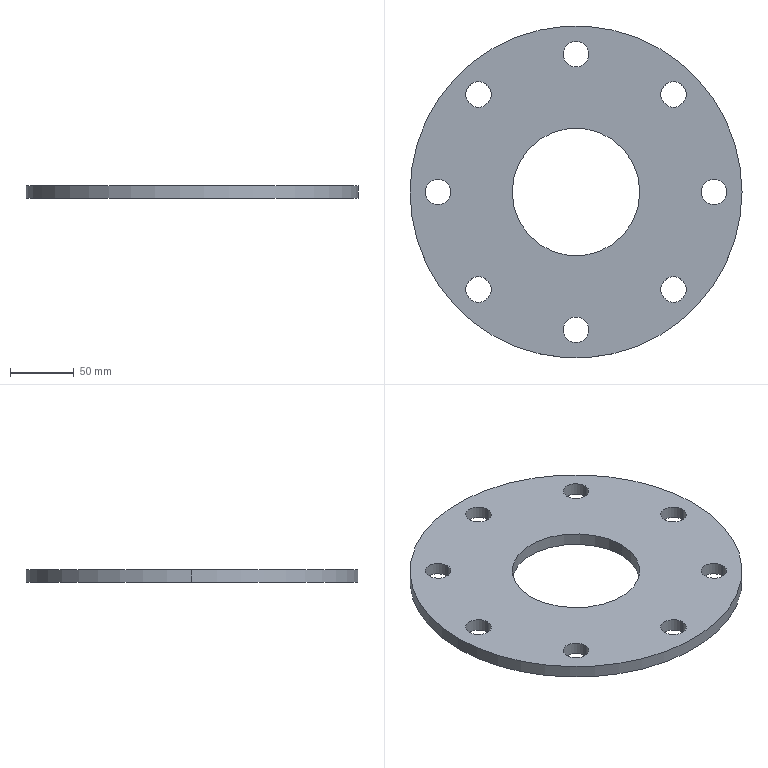Part | SolidWorks | features Extrusion 1, ICE 1 | 1 solid | 22 faces | box 260 x 260 x 10 mm | volume 427257 mm3 | cylinder 20 | plane 2 | commonest cylinder face diameters 20 x16 100 x2 260 x2
STEP:
#1=CARTESIAN_POINT('',(-50.,0.,-5.));
#2=VERTEX_POINT('',#1);
#3=CARTESIAN_POINT('',(50.,0.,-5.));
#4=VERTEX_POINT('',#3);
#5=CARTESIAN_POINT('',(0.,0.,-5.));
#6=DIRECTION('',(0.,0.,1.));
#7=DIRECTION('',(1.,0.,0.));
#8=AXIS2_PLACEMENT_3D('',#5,#6,#7);
#9=CIRCLE('',#8,50.);
#10=EDGE_CURVE('',#2,#4,#9,.T.);
#11=ORIENTED_EDGE('',*,*,#10,.F.);
#12=CARTESIAN_POINT('',(-50.,0.,5.));
#13=VERTEX_POINT('',#12);
#14=CARTESIAN_POINT('',(-50.,0.,-5.));
#15=DIRECTION('',(0.,0.,1.));
#16=VECTOR('',#15,1000.);
#17=LINE('',#14,#16);
#18=EDGE_CURVE('',#2,#13,#17,.T.);
#19=ORIENTED_EDGE('',*,*,#18,.T.);
#20=CARTESIAN_POINT('',(50.,0.,5.));
#21=VERTEX_POINT('',#20);
#22=CARTESIAN_POINT('',(0.,0.,5.));
#23=DIRECTION('',(0.,0.,1.));
#24=DIRECTION('',(1.,0.,0.));
#25=AXIS2_PLACEMENT_3D('',#22,#23,#24);
#26=CIRCLE('',#25,50.);
#27=EDGE_CURVE('',#13,#21,#26,.T.);
#28=ORIENTED_EDGE('',*,*,#27,.T.);
#29=CARTESIAN_POINT('',(50.,0.,-5.));
#30=DIRECTION('',(0.,0.,1.));
#31=VECTOR('',#30,1000.);
#32=LINE('',#29,#31);
#33=EDGE_CURVE('',#4,#21,#32,.T.);
#34=ORIENTED_EDGE('',*,*,#33,.F.);
#35=EDGE_LOOP('',(#11,#19,#28,#34));
#36=FACE_OUTER_BOUND('',#35,.T.);
#37=CARTESIAN_POINT('',(0.,0.,-5.));
#38=DIRECTION('',(0.,0.,1.));
#39=DIRECTION('',(1.,0.,0.));
#40=AXIS2_PLACEMENT_3D('',#37,#38,#39);
#41=CYLINDRICAL_SURFACE('',#40,50.);
#42=ADVANCED_FACE('',(#36),#41,.F.);
#43=CARTESIAN_POINT('',(-86.368,76.368,5.));
#44=VERTEX_POINT('',#43);
#45=CARTESIAN_POINT('',(-66.368,76.368,5.));
#46=VERTEX_POINT('',#45);
#47=CARTESIAN_POINT('',(-76.368,76.368,5.));
#48=DIRECTION('',(0.,0.,1.));
#49=DIRECTION('',(1.,0.,0.));
#50=AXIS2_PLACEMENT_3D('',#47,#48,#49);
#51=CIRCLE('',#50,10.);
#52=EDGE_CURVE('',#44,#46,#51,.T.);
#53=ORIENTED_EDGE('',*,*,#52,.T.);
#54=CARTESIAN_POINT('',(-66.368,76.368,-5.));
#55=VERTEX_POINT('',#54);
#56=CARTESIAN_POINT('',(-66.368,76.368,5.));
#57=DIRECTION('',(0.,0.,-1.));
#58=VECTOR('',#57,1000.);
#59=LINE('',#56,#58);
#60=EDGE_CURVE('',#46,#55,#59,.T.);
#61=ORIENTED_EDGE('',*,*,#60,.T.);
#62=CARTESIAN_POINT('',(-86.368,76.368,-5.));
#63=VERTEX_POINT('',#62);
#64=CARTESIAN_POINT('',(-76.368,76.368,-5.));
#65=DIRECTION('',(0.,0.,1.));
#66=DIRECTION('',(1.,0.,0.));
#67=AXIS2_PLACEMENT_3D('',#64,#65,#66);
#68=CIRCLE('',#67,10.);
#69=EDGE_CURVE('',#63,#55,#68,.T.);
#70=ORIENTED_EDGE('',*,*,#69,.F.);
#71=CARTESIAN_POINT('',(-86.368,76.368,5.));
#72=DIRECTION('',(0.,0.,-1.));
#73=VECTOR('',#72,1000.);
#74=LINE('',#71,#73);
#75=EDGE_CURVE('',#44,#63,#74,.T.);
#76=ORIENTED_EDGE('',*,*,#75,.F.);
#77=EDGE_LOOP('',(#53,#61,#70,#76));
#78=FACE_OUTER_BOUND('',#77,.T.);
#79=CARTESIAN_POINT('',(-76.368,76.368,5.));
#80=DIRECTION('',(0.,0.,-1.));
#81=DIRECTION('',(-1.,0.,0.));
#82=AXIS2_PLACEMENT_3D('',#79,#80,#81);
#83=CYLINDRICAL_SURFACE('',#82,10.);
#84=ADVANCED_FACE('',(#78),#83,.F.);
#85=CARTESIAN_POINT('',(-118.,0.,5.));
#86=VERTEX_POINT('',#85);
#87=CARTESIAN_POINT('',(-98.,0.,5.));
#88=VERTEX_POINT('',#87);
#89=CARTESIAN_POINT('',(-108.,0.,5.));
#90=DIRECTION('',(0.,0.,1.));
#91=DIRECTION('',(1.,0.,0.));
#92=AXIS2_PLACEMENT_3D('',#89,#90,#91);
#93=CIRCLE('',#92,10.);
#94=EDGE_CURVE('',#86,#88,#93,.T.);
#95=ORIENTED_EDGE('',*,*,#94,.T.);
#96=CARTESIAN_POINT('',(-98.,0.,-5.));
#97=VERTEX_POINT('',#96);
#98=CARTESIAN_POINT('',(-98.,0.,5.));
#99=DIRECTION('',(0.,0.,-1.));
#100=VECTOR('',#99,1000.);
#101=LINE('',#98,#100);
#102=EDGE_CURVE('',#88,#97,#101,.T.);
#103=ORIENTED_EDGE('',*,*,#102,.T.);
#104=CARTESIAN_POINT('',(-118.,0.,-5.));
#105=VERTEX_POINT('',#104);
#106=CARTESIAN_POINT('',(-108.,0.,-5.));
#107=DIRECTION('',(0.,0.,1.));
#108=DIRECTION('',(1.,0.,0.));
#109=AXIS2_PLACEMENT_3D('',#106,#107,#108);
#110=CIRCLE('',#109,10.);
#111=EDGE_CURVE('',#105,#97,#110,.T.);
#112=ORIENTED_EDGE('',*,*,#111,.F.);
#113=CARTESIAN_POINT('',(-118.,0.,5.));
#114=DIRECTION('',(0.,0.,-1.));
#115=VECTOR('',#114,1000.);
#116=LINE('',#113,#115);
#117=EDGE_CURVE('',#86,#105,#116,.T.);
#118=ORIENTED_EDGE('',*,*,#117,.F.);
#119=EDGE_LOOP('',(#95,#103,#112,#118));
#120=FACE_OUTER_BOUND('',#119,.T.);
#121=CARTESIAN_POINT('',(-108.,0.,5.));
#122=DIRECTION('',(0.,0.,-1.));
#123=DIRECTION('',(-1.,0.,0.));
#124=AXIS2_PLACEMENT_3D('',#121,#122,#123);
#125=CYLINDRICAL_SURFACE('',#124,10.);
#126=ADVANCED_FACE('',(#120),#125,.F.);
#127=CARTESIAN_POINT('',(-86.368,-76.368,5.));
#128=VERTEX_POINT('',#127);
#129=CARTESIAN_POINT('',(-66.368,-76.368,5.));
#130=VERTEX_POINT('',#129);
#131=CARTESIAN_POINT('',(-76.368,-76.368,5.));
#132=DIRECTION('',(0.,0.,1.));
#133=DIRECTION('',(1.,0.,0.));
#134=AXIS2_PLACEMENT_3D('',#131,#132,#133);
#135=CIRCLE('',#134,10.);
#136=EDGE_CURVE('',#128,#130,#135,.T.);
#137=ORIENTED_EDGE('',*,*,#136,.T.);
#138=CARTESIAN_POINT('',(-66.368,-76.368,-5.));
#139=VERTEX_POINT('',#138);
#140=CARTESIAN_POINT('',(-66.368,-76.368,5.));
#141=DIRECTION('',(0.,0.,-1.));
#142=VECTOR('',#141,1000.);
#143=LINE('',#140,#142);
#144=EDGE_CURVE('',#130,#139,#143,.T.);
#145=ORIENTED_EDGE('',*,*,#144,.T.);
#146=CARTESIAN_POINT('',(-86.368,-76.368,-5.));
#147=VERTEX_POINT('',#146);
#148=CARTESIAN_POINT('',(-76.368,-76.368,-5.));
#149=DIRECTION('',(0.,0.,1.));
#150=DIRECTION('',(1.,0.,0.));
#151=AXIS2_PLACEMENT_3D('',#148,#149,#150);
#152=CIRCLE('',#151,10.);
#153=EDGE_CURVE('',#147,#139,#152,.T.);
#154=ORIENTED_EDGE('',*,*,#153,.F.);
#155=CARTESIAN_POINT('',(-86.368,-76.368,5.));
#156=DIRECTION('',(0.,0.,-1.));
#157=VECTOR('',#156,1000.);
#158=LINE('',#155,#157);
#159=EDGE_CURVE('',#128,#147,#158,.T.);
#160=ORIENTED_EDGE('',*,*,#159,.F.);
#161=EDGE_LOOP('',(#137,#145,#154,#160));
#162=FACE_OUTER_BOUND('',#161,.T.);
#163=CARTESIAN_POINT('',(-76.368,-76.368,5.));
#164=DIRECTION('',(0.,0.,-1.));
#165=DIRECTION('',(-1.,0.,0.));
#166=AXIS2_PLACEMENT_3D('',#163,#164,#165);
#167=CYLINDRICAL_SURFACE('',#166,10.);
#168=ADVANCED_FACE('',(#162),#167,.F.);
#169=CARTESIAN_POINT('',(-10.,-108.,5.));
#170=VERTEX_POINT('',#169);
#171=CARTESIAN_POINT('',(10.,-108.,5.));
#172=VERTEX_POINT('',#171);
#173=CARTESIAN_POINT('',(0.,-108.,5.));
#174=DIRECTION('',(0.,0.,1.));
#175=DIRECTION('',(1.,0.,0.));
#176=AXIS2_PLACEMENT_3D('',#173,#174,#175);
#177=CIRCLE('',#176,10.);
#178=EDGE_CURVE('',#170,#172,#177,.T.);
#179=ORIENTED_EDGE('',*,*,#178,.T.);
#180=CARTESIAN_POINT('',(10.,-108.,-5.));
#181=VERTEX_POINT('',#180);
#182=CARTESIAN_POINT('',(10.,-108.,5.));
#183=DIRECTION('',(0.,0.,-1.));
#184=VECTOR('',#183,1000.);
#185=LINE('',#182,#184);
#186=EDGE_CURVE('',#172,#181,#185,.T.);
#187=ORIENTED_EDGE('',*,*,#186,.T.);
#188=CARTESIAN_POINT('',(-10.,-108.,-5.));
#189=VERTEX_POINT('',#188);
#190=CARTESIAN_POINT('',(0.,-108.,-5.));
#191=DIRECTION('',(0.,0.,1.));
#192=DIRECTION('',(1.,0.,0.));
#193=AXIS2_PLACEMENT_3D('',#190,#191,#192);
#194=CIRCLE('',#193,10.);
#195=EDGE_CURVE('',#189,#181,#194,.T.);
#196=ORIENTED_EDGE('',*,*,#195,.F.);
#197=CARTESIAN_POINT('',(-10.,-108.,5.));
#198=DIRECTION('',(0.,0.,-1.));
#199=VECTOR('',#198,1000.);
#200=LINE('',#197,#199);
#201=EDGE_CURVE('',#170,#189,#200,.T.);
#202=ORIENTED_EDGE('',*,*,#201,.F.);
#203=EDGE_LOOP('',(#179,#187,#196,#202));
#204=FACE_OUTER_BOUND('',#203,.T.);
#205=CARTESIAN_POINT('',(0.,-108.,5.));
#206=DIRECTION('',(0.,0.,-1.));
#207=DIRECTION('',(-1.,0.,0.));
#208=AXIS2_PLACEMENT_3D('',#205,#206,#207);
#209=CYLINDRICAL_SURFACE('',#208,10.);
#210=ADVANCED_FACE('',(#204),#209,.F.);
#211=CARTESIAN_POINT('',(66.368,-76.368,5.));
#212=VERTEX_POINT('',#211);
#213=CARTESIAN_POINT('',(86.368,-76.368,5.));
#214=VERTEX_POINT('',#213);
#215=CARTESIAN_POINT('',(76.368,-76.368,5.));
#216=DIRECTION('',(0.,0.,1.));
#217=DIRECTION('',(1.,0.,0.));
#218=AXIS2_PLACEMENT_3D('',#215,#216,#217);
#219=CIRCLE('',#218,10.);
#220=EDGE_CURVE('',#212,#214,#219,.T.);
#221=ORIENTED_EDGE('',*,*,#220,.T.);
#222=CARTESIAN_POINT('',(86.368,-76.368,-5.));
#223=VERTEX_POINT('',#222);
#224=CARTESIAN_POINT('',(86.368,-76.368,5.));
#225=DIRECTION('',(0.,0.,-1.));
#226=VECTOR('',#225,1000.);
#227=LINE('',#224,#226);
#228=EDGE_CURVE('',#214,#223,#227,.T.);
#229=ORIENTED_EDGE('',*,*,#228,.T.);
#230=CARTESIAN_POINT('',(66.368,-76.368,-5.));
#231=VERTEX_POINT('',#230);
#232=CARTESIAN_POINT('',(76.368,-76.368,-5.));
#233=DIRECTION('',(0.,0.,1.));
#234=DIRECTION('',(1.,0.,0.));
#235=AXIS2_PLACEMENT_3D('',#232,#233,#234);
#236=CIRCLE('',#235,10.);
#237=EDGE_CURVE('',#231,#223,#236,.T.);
#238=ORIENTED_EDGE('',*,*,#237,.F.);
#239=CARTESIAN_POINT('',(66.368,-76.368,5.));
#240=DIRECTION('',(0.,0.,-1.));
#241=VECTOR('',#240,1000.);
#242=LINE('',#239,#241);
#243=EDGE_CURVE('',#212,#231,#242,.T.);
#244=ORIENTED_EDGE('',*,*,#243,.F.);
#245=EDGE_LOOP('',(#221,#229,#238,#244));
#246=FACE_OUTER_BOUND('',#245,.T.);
#247=CARTESIAN_POINT('',(76.368,-76.368,5.));
#248=DIRECTION('',(0.,0.,-1.));
#249=DIRECTION('',(-1.,0.,0.));
#250=AXIS2_PLACEMENT_3D('',#247,#248,#249);
#251=CYLINDRICAL_SURFACE('',#250,10.);
#252=ADVANCED_FACE('',(#246),#251,.F.);
#253=CARTESIAN_POINT('',(98.,0.,5.));
#254=VERTEX_POINT('',#253);
#255=CARTESIAN_POINT('',(118.,0.,5.));
#256=VERTEX_POINT('',#255);
#257=CARTESIAN_POINT('',(108.,0.,5.));
#258=DIRECTION('',(0.,0.,1.));
#259=DIRECTION('',(1.,0.,0.));
#260=AXIS2_PLACEMENT_3D('',#257,#258,#259);
#261=CIRCLE('',#260,10.);
#262=EDGE_CURVE('',#254,#256,#261,.T.);
#263=ORIENTED_EDGE('',*,*,#262,.T.);
#264=CARTESIAN_POINT('',(118.,0.,-5.));
#265=VERTEX_POINT('',#264);
#266=CARTESIAN_POINT('',(118.,0.,5.));
#267=DIRECTION('',(0.,0.,-1.));
#268=VECTOR('',#267,1000.);
#269=LINE('',#266,#268);
#270=EDGE_CURVE('',#256,#265,#269,.T.);
#271=ORIENTED_EDGE('',*,*,#270,.T.);
#272=CARTESIAN_POINT('',(98.,0.,-5.));
#273=VERTEX_POINT('',#272);
#274=CARTESIAN_POINT('',(108.,0.,-5.));
#275=DIRECTION('',(0.,0.,1.));
#276=DIRECTION('',(1.,0.,0.));
#277=AXIS2_PLACEMENT_3D('',#274,#275,#276);
#278=CIRCLE('',#277,10.);
#279=EDGE_CURVE('',#273,#265,#278,.T.);
#280=ORIENTED_EDGE('',*,*,#279,.F.);
#281=CARTESIAN_POINT('',(98.,0.,5.));
#282=DIRECTION('',(0.,0.,-1.));
#283=VECTOR('',#282,1000.);
#284=LINE('',#281,#283);
#285=EDGE_CURVE('',#254,#273,#284,.T.);
#286=ORIENTED_EDGE('',*,*,#285,.F.);
#287=EDGE_LOOP('',(#263,#271,#280,#286));
#288=FACE_OUTER_BOUND('',#287,.T.);
#289=CARTESIAN_POINT('',(108.,0.,5.));
#290=DIRECTION('',(0.,0.,-1.));
#291=DIRECTION('',(-1.,0.,0.));
#292=AXIS2_PLACEMENT_3D('',#289,#290,#291);
#293=CYLINDRICAL_SURFACE('',#292,10.);
#294=ADVANCED_FACE('',(#288),#293,.F.);
#295=CARTESIAN_POINT('',(66.368,76.368,5.));
#296=VERTEX_POINT('',#295);
#297=CARTESIAN_POINT('',(86.368,76.368,5.));
#298=VERTEX_POINT('',#297);
#299=CARTESIAN_POINT('',(76.368,76.368,5.));
#300=DIRECTION('',(0.,0.,1.));
#301=DIRECTION('',(1.,0.,0.));
#302=AXIS2_PLACEMENT_3D('',#299,#300,#301);
#303=CIRCLE('',#302,10.);
#304=EDGE_CURVE('',#296,#298,#303,.T.);
#305=ORIENTED_EDGE('',*,*,#304,.T.);
#306=CARTESIAN_POINT('',(86.368,76.368,-5.));
#307=VERTEX_POINT('',#306);
#308=CARTESIAN_POINT('',(86.368,76.368,5.));
#309=DIRECTION('',(0.,0.,-1.));
#310=VECTOR('',#309,1000.);
#311=LINE('',#308,#310);
#312=EDGE_CURVE('',#298,#307,#311,.T.);
#313=ORIENTED_EDGE('',*,*,#312,.T.);
#314=CARTESIAN_POINT('',(66.368,76.368,-5.));
#315=VERTEX_POINT('',#314);
#316=CARTESIAN_POINT('',(76.368,76.368,-5.));
#317=DIRECTION('',(0.,0.,1.));
#318=DIRECTION('',(1.,0.,0.));
#319=AXIS2_PLACEMENT_3D('',#316,#317,#318);
#320=CIRCLE('',#319,10.);
#321=EDGE_CURVE('',#315,#307,#320,.T.);
#322=ORIENTED_EDGE('',*,*,#321,.F.);
#323=CARTESIAN_POINT('',(66.368,76.368,5.));
#324=DIRECTION('',(0.,0.,-1.));
#325=VECTOR('',#324,1000.);
#326=LINE('',#323,#325);
#327=EDGE_CURVE('',#296,#315,#326,.T.);
#328=ORIENTED_EDGE('',*,*,#327,.F.);
#329=EDGE_LOOP('',(#305,#313,#322,#328));
#330=FACE_OUTER_BOUND('',#329,.T.);
#331=CARTESIAN_POINT('',(76.368,76.368,5.));
#332=DIRECTION('',(0.,0.,-1.));
#333=DIRECTION('',(-1.,0.,0.));
#334=AXIS2_PLACEMENT_3D('',#331,#332,#333);
#335=CYLINDRICAL_SURFACE('',#334,10.);
#336=ADVANCED_FACE('',(#330),#335,.F.);
#337=CARTESIAN_POINT('',(-10.,108.,5.));
#338=VERTEX_POINT('',#337);
#339=CARTESIAN_POINT('',(10.,108.,5.));
#340=VERTEX_POINT('',#339);
#341=CARTESIAN_POINT('',(0.,108.,5.));
#342=DIRECTION('',(0.,0.,1.));
#343=DIRECTION('',(1.,0.,0.));
#344=AXIS2_PLACEMENT_3D('',#341,#342,#343);
#345=CIRCLE('',#344,10.);
#346=EDGE_CURVE('',#338,#340,#345,.T.);
#347=ORIENTED_EDGE('',*,*,#346,.T.);
#348=CARTESIAN_POINT('',(10.,108.,-5.));
#349=VERTEX_POINT('',#348);
#350=CARTESIAN_POINT('',(10.,108.,5.));
#351=DIRECTION('',(0.,0.,-1.));
#352=VECTOR('',#351,1000.);
#353=LINE('',#350,#352);
#354=EDGE_CURVE('',#340,#349,#353,.T.);
#355=ORIENTED_EDGE('',*,*,#354,.T.);
#356=CARTESIAN_POINT('',(-10.,108.,-5.));
#357=VERTEX_POINT('',#356);
#358=CARTESIAN_POINT('',(0.,108.,-5.));
#359=DIRECTION('',(0.,0.,1.));
#360=DIRECTION('',(1.,0.,0.));
#361=AXIS2_PLACEMENT_3D('',#358,#359,#360);
#362=CIRCLE('',#361,10.);
#363=EDGE_CURVE('',#357,#349,#362,.T.);
#364=ORIENTED_EDGE('',*,*,#363,.F.);
#365=CARTESIAN_POINT('',(-10.,108.,5.));
#366=DIRECTION('',(0.,0.,-1.));
#367=VECTOR('',#366,1000.);
#368=LINE('',#365,#367);
#369=EDGE_CURVE('',#338,#357,#368,.T.);
#370=ORIENTED_EDGE('',*,*,#369,.F.);
#371=EDGE_LOOP('',(#347,#355,#364,#370));
#372=FACE_OUTER_BOUND('',#371,.T.);
#373=CARTESIAN_POINT('',(0.,108.,5.));
#374=DIRECTION('',(0.,0.,-1.));
#375=DIRECTION('',(-1.,0.,0.));
#376=AXIS2_PLACEMENT_3D('',#373,#374,#375);
#377=CYLINDRICAL_SURFACE('',#376,10.);
#378=ADVANCED_FACE('',(#372),#377,.F.);
#379=CARTESIAN_POINT('',(130.,0.,5.));
#380=VERTEX_POINT('',#379);
#381=CARTESIAN_POINT('',(-130.,0.,5.));
#382=VERTEX_POINT('',#381);
#383=CARTESIAN_POINT('',(0.,0.,5.));
#384=DIRECTION('',(0.,0.,1.));
#385=DIRECTION('',(1.,0.,0.));
#386=AXIS2_PLACEMENT_3D('',#383,#384,#385);
#387=CIRCLE('',#386,130.);
#388=EDGE_CURVE('',#380,#382,#387,.T.);
#389=ORIENTED_EDGE('',*,*,#388,.F.);
#390=CARTESIAN_POINT('',(130.,0.,-5.));
#391=VERTEX_POINT('',#390);
#392=CARTESIAN_POINT('',(130.,0.,5.));
#393=DIRECTION('',(0.,0.,-1.));
#394=VECTOR('',#393,1000.);
#395=LINE('',#392,#394);
#396=EDGE_CURVE('',#380,#391,#395,.T.);
#397=ORIENTED_EDGE('',*,*,#396,.T.);
#398=CARTESIAN_POINT('',(-130.,0.,-5.));
#399=VERTEX_POINT('',#398);
#400=CARTESIAN_POINT('',(0.,0.,-5.));
#401=DIRECTION('',(0.,0.,1.));
#402=DIRECTION('',(1.,0.,0.));
#403=AXIS2_PLACEMENT_3D('',#400,#401,#402);
#404=CIRCLE('',#403,130.);
#405=EDGE_CURVE('',#391,#399,#404,.T.);
#406=ORIENTED_EDGE('',*,*,#405,.T.);
#407=CARTESIAN_POINT('',(-130.,0.,5.));
#408=DIRECTION('',(0.,0.,-1.));
#409=VECTOR('',#408,1000.);
#410=LINE('',#407,#409);
#411=EDGE_CURVE('',#382,#399,#410,.T.);
#412=ORIENTED_EDGE('',*,*,#411,.F.);
#413=EDGE_LOOP('',(#389,#397,#406,#412));
#414=FACE_OUTER_BOUND('',#413,.T.);
#415=CARTESIAN_POINT('',(0.,0.,5.));
#416=DIRECTION('',(0.,0.,-1.));
#417=DIRECTION('',(-1.,0.,0.));
#418=AXIS2_PLACEMENT_3D('',#415,#416,#417);
#419=CYLINDRICAL_SURFACE('',#418,130.);
#420=ADVANCED_FACE('',(#414),#419,.T.);
#421=CARTESIAN_POINT('',(0.,0.,5.));
#422=DIRECTION('',(0.,0.,1.));
#423=DIRECTION('',(1.,0.,0.));
#424=AXIS2_PLACEMENT_3D('',#421,#422,#423);
#425=CIRCLE('',#424,50.);
#426=EDGE_CURVE('',#21,#13,#425,.T.);
#427=ORIENTED_EDGE('',*,*,#426,.F.);
#428=ORIENTED_EDGE('',*,*,#27,.F.);
#429=EDGE_LOOP('',(#427,#428));
#430=FACE_BOUND('',#429,.T.);
#431=ORIENTED_EDGE('',*,*,#94,.F.);
#432=CARTESIAN_POINT('',(-108.,0.,5.));
#433=DIRECTION('',(0.,0.,1.));
#434=DIRECTION('',(1.,0.,0.));
#435=AXIS2_PLACEMENT_3D('',#432,#433,#434);
#436=CIRCLE('',#435,10.);
#437=EDGE_CURVE('',#88,#86,#436,.T.);
#438=ORIENTED_EDGE('',*,*,#437,.F.);
#439=EDGE_LOOP('',(#431,#438));
#440=FACE_BOUND('',#439,.T.);
#441=ORIENTED_EDGE('',*,*,#178,.F.);
#442=CARTESIAN_POINT('',(0.,-108.,5.));
#443=DIRECTION('',(0.,0.,1.));
#444=DIRECTION('',(1.,0.,0.));
#445=AXIS2_PLACEMENT_3D('',#442,#443,#444);
#446=CIRCLE('',#445,10.);
#447=EDGE_CURVE('',#172,#170,#446,.T.);
#448=ORIENTED_EDGE('',*,*,#447,.F.);
#449=EDGE_LOOP('',(#441,#448));
#450=FACE_BOUND('',#449,.T.);
#451=ORIENTED_EDGE('',*,*,#262,.F.);
#452=CARTESIAN_POINT('',(108.,0.,5.));
#453=DIRECTION('',(0.,0.,1.));
#454=DIRECTION('',(1.,0.,0.));
#455=AXIS2_PLACEMENT_3D('',#452,#453,#454);
#456=CIRCLE('',#455,10.);
#457=EDGE_CURVE('',#256,#254,#456,.T.);
#458=ORIENTED_EDGE('',*,*,#457,.F.);
#459=EDGE_LOOP('',(#451,#458));
#460=FACE_BOUND('',#459,.T.);
#461=ORIENTED_EDGE('',*,*,#346,.F.);
#462=CARTESIAN_POINT('',(0.,108.,5.));
#463=DIRECTION('',(0.,0.,1.));
#464=DIRECTION('',(1.,0.,0.));
#465=AXIS2_PLACEMENT_3D('',#462,#463,#464);
#466=CIRCLE('',#465,10.);
#467=EDGE_CURVE('',#340,#338,#466,.T.);
#468=ORIENTED_EDGE('',*,*,#467,.F.);
#469=EDGE_LOOP('',(#461,#468));
#470=FACE_BOUND('',#469,.T.);
#471=CARTESIAN_POINT('',(0.,0.,5.));
#472=DIRECTION('',(0.,0.,1.));
#473=DIRECTION('',(1.,0.,0.));
#474=AXIS2_PLACEMENT_3D('',#471,#472,#473);
#475=CIRCLE('',#474,130.);
#476=EDGE_CURVE('',#382,#380,#475,.T.);
#477=ORIENTED_EDGE('',*,*,#476,.T.);
#478=ORIENTED_EDGE('',*,*,#388,.T.);
#479=EDGE_LOOP('',(#477,#478));
#480=FACE_OUTER_BOUND('',#479,.T.);
#481=ORIENTED_EDGE('',*,*,#304,.F.);
#482=CARTESIAN_POINT('',(76.368,76.368,5.));
#483=DIRECTION('',(0.,0.,1.));
#484=DIRECTION('',(1.,0.,0.));
#485=AXIS2_PLACEMENT_3D('',#482,#483,#484);
#486=CIRCLE('',#485,10.);
#487=EDGE_CURVE('',#298,#296,#486,.T.);
#488=ORIENTED_EDGE('',*,*,#487,.F.);
#489=EDGE_LOOP('',(#481,#488));
#490=FACE_BOUND('',#489,.T.);
#491=ORIENTED_EDGE('',*,*,#220,.F.);
#492=CARTESIAN_POINT('',(76.368,-76.368,5.));
#493=DIRECTION('',(0.,0.,1.));
#494=DIRECTION('',(1.,0.,0.));
#495=AXIS2_PLACEMENT_3D('',#492,#493,#494);
#496=CIRCLE('',#495,10.);
#497=EDGE_CURVE('',#214,#212,#496,.T.);
#498=ORIENTED_EDGE('',*,*,#497,.F.);
#499=EDGE_LOOP('',(#491,#498));
#500=FACE_BOUND('',#499,.T.);
#501=ORIENTED_EDGE('',*,*,#136,.F.);
#502=CARTESIAN_POINT('',(-76.368,-76.368,5.));
#503=DIRECTION('',(0.,0.,1.));
#504=DIRECTION('',(1.,0.,0.));
#505=AXIS2_PLACEMENT_3D('',#502,#503,#504);
#506=CIRCLE('',#505,10.);
#507=EDGE_CURVE('',#130,#128,#506,.T.);
#508=ORIENTED_EDGE('',*,*,#507,.F.);
#509=EDGE_LOOP('',(#501,#508));
#510=FACE_BOUND('',#509,.T.);
#511=ORIENTED_EDGE('',*,*,#52,.F.);
#512=CARTESIAN_POINT('',(-76.368,76.368,5.));
#513=DIRECTION('',(0.,0.,1.));
#514=DIRECTION('',(1.,0.,0.));
#515=AXIS2_PLACEMENT_3D('',#512,#513,#514);
#516=CIRCLE('',#515,10.);
#517=EDGE_CURVE('',#46,#44,#516,.T.);
#518=ORIENTED_EDGE('',*,*,#517,.F.);
#519=EDGE_LOOP('',(#511,#518));
#520=FACE_BOUND('',#519,.T.);
#521=CARTESIAN_POINT('',(0.,0.,5.));
#522=DIRECTION('',(0.,0.,1.));
#523=DIRECTION('',(1.,0.,0.));
#524=AXIS2_PLACEMENT_3D('',#521,#522,#523);
#525=PLANE('',#524);
#526=ADVANCED_FACE('',(#430,#440,#450,#460,#470,#480,#490,#500,#510,#520),#525,.T.);
#527=CARTESIAN_POINT('',(0.,0.,-5.));
#528=DIRECTION('',(0.,0.,1.));
#529=DIRECTION('',(1.,0.,0.));
#530=AXIS2_PLACEMENT_3D('',#527,#528,#529);
#531=CIRCLE('',#530,50.);
#532=EDGE_CURVE('',#4,#2,#531,.T.);
#533=ORIENTED_EDGE('',*,*,#532,.T.);
#534=ORIENTED_EDGE('',*,*,#10,.T.);
#535=EDGE_LOOP('',(#533,#534));
#536=FACE_BOUND('',#535,.T.);
#537=CARTESIAN_POINT('',(0.,0.,-5.));
#538=DIRECTION('',(0.,0.,1.));
#539=DIRECTION('',(1.,0.,0.));
#540=AXIS2_PLACEMENT_3D('',#537,#538,#539);
#541=CIRCLE('',#540,130.);
#542=EDGE_CURVE('',#399,#391,#541,.T.);
#543=ORIENTED_EDGE('',*,*,#542,.F.);
#544=ORIENTED_EDGE('',*,*,#405,.F.);
#545=EDGE_LOOP('',(#543,#544));
#546=FACE_OUTER_BOUND('',#545,.T.);
#547=ORIENTED_EDGE('',*,*,#363,.T.);
#548=CARTESIAN_POINT('',(0.,108.,-5.));
#549=DIRECTION('',(0.,0.,1.));
#550=DIRECTION('',(1.,0.,0.));
#551=AXIS2_PLACEMENT_3D('',#548,#549,#550);
#552=CIRCLE('',#551,10.);
#553=EDGE_CURVE('',#349,#357,#552,.T.);
#554=ORIENTED_EDGE('',*,*,#553,.T.);
#555=EDGE_LOOP('',(#547,#554));
#556=FACE_BOUND('',#555,.T.);
#557=ORIENTED_EDGE('',*,*,#321,.T.);
#558=CARTESIAN_POINT('',(76.368,76.368,-5.));
#559=DIRECTION('',(0.,0.,1.));
#560=DIRECTION('',(1.,0.,0.));
#561=AXIS2_PLACEMENT_3D('',#558,#559,#560);
#562=CIRCLE('',#561,10.);
#563=EDGE_CURVE('',#307,#315,#562,.T.);
#564=ORIENTED_EDGE('',*,*,#563,.T.);
#565=EDGE_LOOP('',(#557,#564));
#566=FACE_BOUND('',#565,.T.);
#567=ORIENTED_EDGE('',*,*,#279,.T.);
#568=CARTESIAN_POINT('',(108.,0.,-5.));
#569=DIRECTION('',(0.,0.,1.));
#570=DIRECTION('',(1.,0.,0.));
#571=AXIS2_PLACEMENT_3D('',#568,#569,#570);
#572=CIRCLE('',#571,10.);
#573=EDGE_CURVE('',#265,#273,#572,.T.);
#574=ORIENTED_EDGE('',*,*,#573,.T.);
#575=EDGE_LOOP('',(#567,#574));
#576=FACE_BOUND('',#575,.T.);
#577=ORIENTED_EDGE('',*,*,#237,.T.);
#578=CARTESIAN_POINT('',(76.368,-76.368,-5.));
#579=DIRECTION('',(0.,0.,1.));
#580=DIRECTION('',(1.,0.,0.));
#581=AXIS2_PLACEMENT_3D('',#578,#579,#580);
#582=CIRCLE('',#581,10.);
#583=EDGE_CURVE('',#223,#231,#582,.T.);
#584=ORIENTED_EDGE('',*,*,#583,.T.);
#585=EDGE_LOOP('',(#577,#584));
#586=FACE_BOUND('',#585,.T.);
#587=ORIENTED_EDGE('',*,*,#195,.T.);
#588=CARTESIAN_POINT('',(0.,-108.,-5.));
#589=DIRECTION('',(0.,0.,1.));
#590=DIRECTION('',(1.,0.,0.));
#591=AXIS2_PLACEMENT_3D('',#588,#589,#590);
#592=CIRCLE('',#591,10.);
#593=EDGE_CURVE('',#181,#189,#592,.T.);
#594=ORIENTED_EDGE('',*,*,#593,.T.);
#595=EDGE_LOOP('',(#587,#594));
#596=FACE_BOUND('',#595,.T.);
#597=ORIENTED_EDGE('',*,*,#153,.T.);
#598=CARTESIAN_POINT('',(-76.368,-76.368,-5.));
#599=DIRECTION('',(0.,0.,1.));
#600=DIRECTION('',(1.,0.,0.));
#601=AXIS2_PLACEMENT_3D('',#598,#599,#600);
#602=CIRCLE('',#601,10.);
#603=EDGE_CURVE('',#139,#147,#602,.T.);
#604=ORIENTED_EDGE('',*,*,#603,.T.);
#605=EDGE_LOOP('',(#597,#604));
#606=FACE_BOUND('',#605,.T.);
#607=ORIENTED_EDGE('',*,*,#111,.T.);
#608=CARTESIAN_POINT('',(-108.,0.,-5.));
#609=DIRECTION('',(0.,0.,1.));
#610=DIRECTION('',(1.,0.,0.));
#611=AXIS2_PLACEMENT_3D('',#608,#609,#610);
#612=CIRCLE('',#611,10.);
#613=EDGE_CURVE('',#97,#105,#612,.T.);
#614=ORIENTED_EDGE('',*,*,#613,.T.);
#615=EDGE_LOOP('',(#607,#614));
#616=FACE_BOUND('',#615,.T.);
#617=ORIENTED_EDGE('',*,*,#69,.T.);
#618=CARTESIAN_POINT('',(-76.368,76.368,-5.));
#619=DIRECTION('',(0.,0.,1.));
#620=DIRECTION('',(1.,0.,0.));
#621=AXIS2_PLACEMENT_3D('',#618,#619,#620);
#622=CIRCLE('',#621,10.);
#623=EDGE_CURVE('',#55,#63,#622,.T.);
#624=ORIENTED_EDGE('',*,*,#623,.T.);
#625=EDGE_LOOP('',(#617,#624));
#626=FACE_BOUND('',#625,.T.);
#627=CARTESIAN_POINT('',(0.,0.,-5.));
#628=DIRECTION('',(0.,0.,1.));
#629=DIRECTION('',(1.,0.,0.));
#630=AXIS2_PLACEMENT_3D('',#627,#628,#629);
#631=PLANE('',#630);
#632=ADVANCED_FACE('',(#536,#546,#556,#566,#576,#586,#596,#606,#616,#626),#631,.F.);
#633=ORIENTED_EDGE('',*,*,#396,.F.);
#634=ORIENTED_EDGE('',*,*,#476,.F.);
#635=ORIENTED_EDGE('',*,*,#411,.T.);
#636=ORIENTED_EDGE('',*,*,#542,.T.);
#637=EDGE_LOOP('',(#633,#634,#635,#636));
#638=FACE_OUTER_BOUND('',#637,.T.);
#639=CARTESIAN_POINT('',(0.,0.,5.));
#640=DIRECTION('',(0.,0.,-1.));
#641=DIRECTION('',(-1.,0.,0.));
#642=AXIS2_PLACEMENT_3D('',#639,#640,#641);
#643=CYLINDRICAL_SURFACE('',#642,130.);
#644=ADVANCED_FACE('',(#638),#643,.T.);
#645=ORIENTED_EDGE('',*,*,#354,.F.);
#646=ORIENTED_EDGE('',*,*,#467,.T.);
#647=ORIENTED_EDGE('',*,*,#369,.T.);
#648=ORIENTED_EDGE('',*,*,#553,.F.);
#649=EDGE_LOOP('',(#645,#646,#647,#648));
#650=FACE_OUTER_BOUND('',#649,.T.);
#651=CARTESIAN_POINT('',(0.,108.,5.));
#652=DIRECTION('',(0.,0.,-1.));
#653=DIRECTION('',(-1.,0.,0.));
#654=AXIS2_PLACEMENT_3D('',#651,#652,#653);
#655=CYLINDRICAL_SURFACE('',#654,10.);
#656=ADVANCED_FACE('',(#650),#655,.F.);
#657=ORIENTED_EDGE('',*,*,#312,.F.);
#658=ORIENTED_EDGE('',*,*,#487,.T.);
#659=ORIENTED_EDGE('',*,*,#327,.T.);
#660=ORIENTED_EDGE('',*,*,#563,.F.);
#661=EDGE_LOOP('',(#657,#658,#659,#660));
#662=FACE_OUTER_BOUND('',#661,.T.);
#663=CARTESIAN_POINT('',(76.368,76.368,5.));
#664=DIRECTION('',(0.,0.,-1.));
#665=DIRECTION('',(-1.,0.,0.));
#666=AXIS2_PLACEMENT_3D('',#663,#664,#665);
#667=CYLINDRICAL_SURFACE('',#666,10.);
#668=ADVANCED_FACE('',(#662),#667,.F.);
#669=ORIENTED_EDGE('',*,*,#270,.F.);
#670=ORIENTED_EDGE('',*,*,#457,.T.);
#671=ORIENTED_EDGE('',*,*,#285,.T.);
#672=ORIENTED_EDGE('',*,*,#573,.F.);
#673=EDGE_LOOP('',(#669,#670,#671,#672));
#674=FACE_OUTER_BOUND('',#673,.T.);
#675=CARTESIAN_POINT('',(108.,0.,5.));
#676=DIRECTION('',(0.,0.,-1.));
#677=DIRECTION('',(-1.,0.,0.));
#678=AXIS2_PLACEMENT_3D('',#675,#676,#677);
#679=CYLINDRICAL_SURFACE('',#678,10.);
#680=ADVANCED_FACE('',(#674),#679,.F.);
#681=ORIENTED_EDGE('',*,*,#228,.F.);
#682=ORIENTED_EDGE('',*,*,#497,.T.);
#683=ORIENTED_EDGE('',*,*,#243,.T.);
#684=ORIENTED_EDGE('',*,*,#583,.F.);
#685=EDGE_LOOP('',(#681,#682,#683,#684));
#686=FACE_OUTER_BOUND('',#685,.T.);
#687=CARTESIAN_POINT('',(76.368,-76.368,5.));
#688=DIRECTION('',(0.,0.,-1.));
#689=DIRECTION('',(-1.,0.,0.));
#690=AXIS2_PLACEMENT_3D('',#687,#688,#689);
#691=CYLINDRICAL_SURFACE('',#690,10.);
#692=ADVANCED_FACE('',(#686),#691,.F.);
#693=ORIENTED_EDGE('',*,*,#186,.F.);
#694=ORIENTED_EDGE('',*,*,#447,.T.);
#695=ORIENTED_EDGE('',*,*,#201,.T.);
#696=ORIENTED_EDGE('',*,*,#593,.F.);
#697=EDGE_LOOP('',(#693,#694,#695,#696));
#698=FACE_OUTER_BOUND('',#697,.T.);
#699=CARTESIAN_POINT('',(0.,-108.,5.));
#700=DIRECTION('',(0.,0.,-1.));
#701=DIRECTION('',(-1.,0.,0.));
#702=AXIS2_PLACEMENT_3D('',#699,#700,#701);
#703=CYLINDRICAL_SURFACE('',#702,10.);
#704=ADVANCED_FACE('',(#698),#703,.F.);
#705=ORIENTED_EDGE('',*,*,#144,.F.);
#706=ORIENTED_EDGE('',*,*,#507,.T.);
#707=ORIENTED_EDGE('',*,*,#159,.T.);
#708=ORIENTED_EDGE('',*,*,#603,.F.);
#709=EDGE_LOOP('',(#705,#706,#707,#708));
#710=FACE_OUTER_BOUND('',#709,.T.);
#711=CARTESIAN_POINT('',(-76.368,-76.368,5.));
#712=DIRECTION('',(0.,0.,-1.));
#713=DIRECTION('',(-1.,0.,0.));
#714=AXIS2_PLACEMENT_3D('',#711,#712,#713);
#715=CYLINDRICAL_SURFACE('',#714,10.);
#716=ADVANCED_FACE('',(#710),#715,.F.);
#717=ORIENTED_EDGE('',*,*,#102,.F.);
#718=ORIENTED_EDGE('',*,*,#437,.T.);
#719=ORIENTED_EDGE('',*,*,#117,.T.);
#720=ORIENTED_EDGE('',*,*,#613,.F.);
#721=EDGE_LOOP('',(#717,#718,#719,#720));
#722=FACE_OUTER_BOUND('',#721,.T.);
#723=CARTESIAN_POINT('',(-108.,0.,5.));
#724=DIRECTION('',(0.,0.,-1.));
#725=DIRECTION('',(-1.,0.,0.));
#726=AXIS2_PLACEMENT_3D('',#723,#724,#725);
#727=CYLINDRICAL_SURFACE('',#726,10.);
#728=ADVANCED_FACE('',(#722),#727,.F.);
#729=ORIENTED_EDGE('',*,*,#60,.F.);
#730=ORIENTED_EDGE('',*,*,#517,.T.);
#731=ORIENTED_EDGE('',*,*,#75,.T.);
#732=ORIENTED_EDGE('',*,*,#623,.F.);
#733=EDGE_LOOP('',(#729,#730,#731,#732));
#734=FACE_OUTER_BOUND('',#733,.T.);
#735=CARTESIAN_POINT('',(-76.368,76.368,5.));
#736=DIRECTION('',(0.,0.,-1.));
#737=DIRECTION('',(-1.,0.,0.));
#738=AXIS2_PLACEMENT_3D('',#735,#736,#737);
#739=CYLINDRICAL_SURFACE('',#738,10.);
#740=ADVANCED_FACE('',(#734),#739,.F.);
#741=ORIENTED_EDGE('',*,*,#18,.F.);
#742=ORIENTED_EDGE('',*,*,#532,.F.);
#743=ORIENTED_EDGE('',*,*,#33,.T.);
#744=ORIENTED_EDGE('',*,*,#426,.T.);
#745=EDGE_LOOP('',(#741,#742,#743,#744));
#746=FACE_OUTER_BOUND('',#745,.T.);
#747=CARTESIAN_POINT('',(0.,0.,-5.));
#748=DIRECTION('',(0.,0.,1.));
#749=DIRECTION('',(1.,0.,0.));
#750=AXIS2_PLACEMENT_3D('',#747,#748,#749);
#751=CYLINDRICAL_SURFACE('',#750,50.);
#752=ADVANCED_FACE('',(#746),#751,.F.);
#753=CLOSED_SHELL('',(#42,#84,#126,#168,#210,#252,#294,#336,#378,#420,#526,#632,#644,#656,#668,#680,#692,#704,#716,#728,#740,#752));
#754=MANIFOLD_SOLID_BREP('',#753);
#755=CARTESIAN_POINT('',(0.,0.,0.));
#756=DIRECTION('',(0.,0.,1.));
#757=DIRECTION('',(1.,0.,0.));
#758=AXIS2_PLACEMENT_3D('',#755,#756,#757);
#759=(LENGTH_UNIT()NAMED_UNIT(*)SI_UNIT(.MILLI.,.METRE.));
#760=UNCERTAINTY_MEASURE_WITH_UNIT(LENGTH_MEASURE(0.00001),#759,'','');
#761=(NAMED_UNIT(*)PLANE_ANGLE_UNIT()SI_UNIT($,.RADIAN.));
#762=(NAMED_UNIT(*)SI_UNIT($,.STERADIAN.)SOLID_ANGLE_UNIT());
#763=(GEOMETRIC_REPRESENTATION_CONTEXT(3)GLOBAL_UNCERTAINTY_ASSIGNED_CONTEXT((#760))GLOBAL_UNIT_ASSIGNED_CONTEXT((#759,#761,#762))REPRESENTATION_CONTEXT('',''));
#764=ADVANCED_BREP_SHAPE_REPRESENTATION('',(#754,#758),#763);